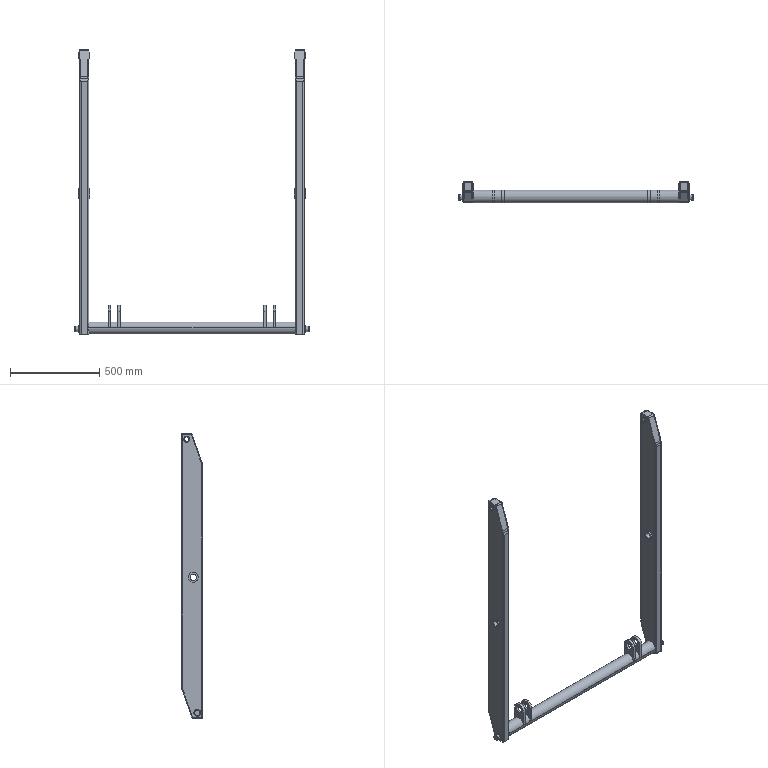Part | STEP file | BT2022003-01-06 Scissor beam B_Default<Machined> | 17 solids | 232 faces | box 1311 x 120 x 1590 mm | volume 5354127 mm3 | cylinder 116 | plane 108 | cone 8 | commonest cylinder face diameters 8 x24 20 x12 34 x12 55 x12 71 x10 16 x8